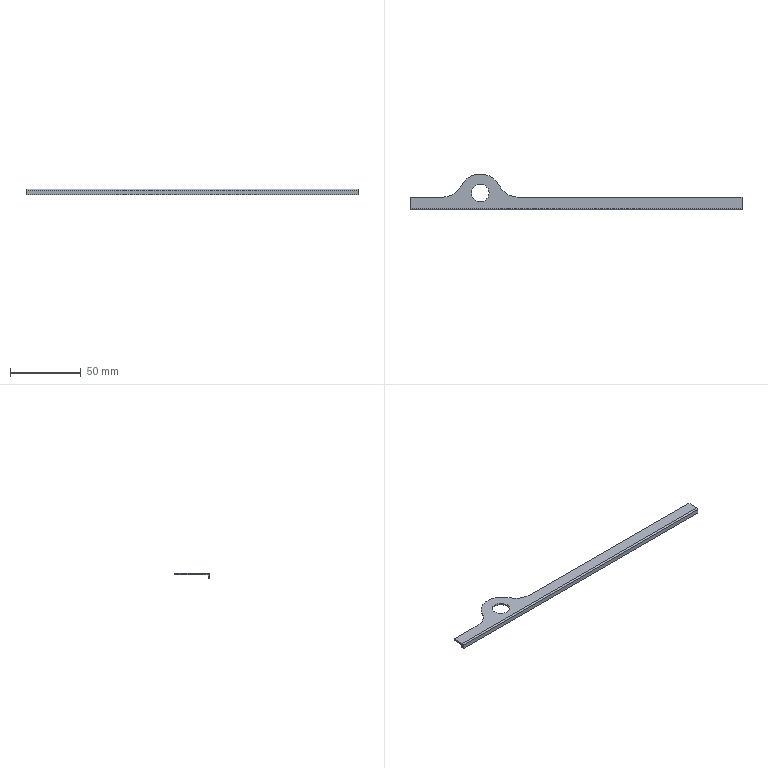Part | STEP file | gslz 2016.10.28-13_id1198_x_t | 1 solid | 14 faces | box 235 x 25.5 x 4 mm | volume 3805 mm3 | plane 9 | cylinder 5 | commonest cylinder face diameters 30 x3 2 x1 12.3 x1
STEP:
#1=CARTESIAN_POINT('',(0.,0.,0.));
#2=DIRECTION('',(0.,0.,1.));
#3=DIRECTION('',(1.,0.,0.));
#4=AXIS2_PLACEMENT_3D('',#1,#2,#3);
#5=CARTESIAN_POINT('',(1039.237,-257.,1.25));
#6=VERTEX_POINT('',#5);
#7=CARTESIAN_POINT('',(1197.655,-257.,1.25));
#8=VERTEX_POINT('',#7);
#9=CARTESIAN_POINT('',(-1199.517,-257.,1.25));
#10=DIRECTION('',(1.,0.,0.));
#11=VECTOR('',#10,1.);
#12=LINE('',#9,#11);
#13=CARTESIAN_POINT('',(1040.731,-257.,2.5));
#14=DIRECTION('',(0.,1.,0.));
#15=DIRECTION('',(-1.,0.,0.));
#16=AXIS2_PLACEMENT_3D('',#13,#14,#15);
#17=PLANE('',#16);
#18=CARTESIAN_POINT('',(2240.248,-1.25));
#19=DIRECTION('',(-1.,0.));
#20=VECTOR('',#19,1.);
#21=LINE('',#18,#20);
#22=(GEOMETRIC_REPRESENTATION_CONTEXT(2)PARAMETRIC_REPRESENTATION_CONTEXT()REPRESENTATION_CONTEXT('',''));
#23=DEFINITIONAL_REPRESENTATION('',(#21),#22);
#24=PCURVE('',#17,#23);
#25=CARTESIAN_POINT('',(-1199.517,-331.067,1.25));
#26=DIRECTION('',(0.,0.,1.));
#27=DIRECTION('',(-1.,0.,0.));
#28=AXIS2_PLACEMENT_3D('',#25,#26,#27);
#29=PLANE('',#28);
#30=CARTESIAN_POINT('',(0.,-74.067));
#31=DIRECTION('',(-1.,0.));
#32=VECTOR('',#31,1.);
#33=LINE('',#30,#32);
#34=(GEOMETRIC_REPRESENTATION_CONTEXT(2)PARAMETRIC_REPRESENTATION_CONTEXT()REPRESENTATION_CONTEXT('',''));
#35=DEFINITIONAL_REPRESENTATION('',(#33),#34);
#36=PCURVE('',#29,#35);
#37=SURFACE_CURVE('',#12,(#24,#36),.PCURVE_S1.);
#38=EDGE_CURVE('',#6,#8,#37,.T.);
#39=ORIENTED_EDGE('',*,*,#38,.T.);
#40=CARTESIAN_POINT('',(1197.655,-257.,0.));
#41=VERTEX_POINT('',#40);
#42=CARTESIAN_POINT('',(1197.655,-257.,2.5));
#43=DIRECTION('',(0.,0.,-1.));
#44=VECTOR('',#43,1.);
#45=LINE('',#42,#44);
#46=CARTESIAN_POINT('',(-156.924,0.));
#47=DIRECTION('',(0.,-1.));
#48=VECTOR('',#47,1.);
#49=LINE('',#46,#48);
#50=(GEOMETRIC_REPRESENTATION_CONTEXT(2)PARAMETRIC_REPRESENTATION_CONTEXT()REPRESENTATION_CONTEXT('',''));
#51=DEFINITIONAL_REPRESENTATION('',(#49),#50);
#52=PCURVE('',#17,#51);
#53=CARTESIAN_POINT('',(1197.655,-261.5,-0.75));
#54=DIRECTION('',(1.,0.,0.));
#55=DIRECTION('',(0.,0.,-1.));
#56=AXIS2_PLACEMENT_3D('',#53,#54,#55);
#57=PLANE('',#56);
#58=CARTESIAN_POINT('',(-3.25,4.5));
#59=DIRECTION('',(1.,0.));
#60=VECTOR('',#59,1.);
#61=LINE('',#58,#60);
#62=(GEOMETRIC_REPRESENTATION_CONTEXT(2)PARAMETRIC_REPRESENTATION_CONTEXT()REPRESENTATION_CONTEXT('',''));
#63=DEFINITIONAL_REPRESENTATION('',(#61),#62);
#64=PCURVE('',#57,#63);
#65=SURFACE_CURVE('',#45,(#52,#64),.PCURVE_S1.);
#66=EDGE_CURVE('',#8,#41,#65,.T.);
#67=ORIENTED_EDGE('',*,*,#66,.T.);
#68=CARTESIAN_POINT('',(1039.237,-257.,0.));
#69=VERTEX_POINT('',#68);
#70=CARTESIAN_POINT('',(1040.731,-257.,0.));
#71=DIRECTION('',(-1.,0.,0.));
#72=VECTOR('',#71,1.);
#73=LINE('',#70,#72);
#74=CARTESIAN_POINT('',(0.,-2.5));
#75=DIRECTION('',(1.,0.));
#76=VECTOR('',#75,1.);
#77=LINE('',#74,#76);
#78=(GEOMETRIC_REPRESENTATION_CONTEXT(2)PARAMETRIC_REPRESENTATION_CONTEXT()REPRESENTATION_CONTEXT('',''));
#79=DEFINITIONAL_REPRESENTATION('',(#77),#78);
#80=PCURVE('',#17,#79);
#81=CARTESIAN_POINT('',(-1199.517,-331.067,0.));
#82=DIRECTION('',(0.,0.,1.));
#83=DIRECTION('',(-1.,0.,0.));
#84=AXIS2_PLACEMENT_3D('',#81,#82,#83);
#85=PLANE('',#84);
#86=CARTESIAN_POINT('',(-2240.248,-74.067));
#87=DIRECTION('',(1.,0.));
#88=VECTOR('',#87,1.);
#89=LINE('',#86,#88);
#90=(GEOMETRIC_REPRESENTATION_CONTEXT(2)PARAMETRIC_REPRESENTATION_CONTEXT()REPRESENTATION_CONTEXT('',''));
#91=DEFINITIONAL_REPRESENTATION('',(#89),#90);
#92=PCURVE('',#85,#91);
#93=SURFACE_CURVE('',#73,(#80,#92),.PCURVE_S1.);
#94=EDGE_CURVE('',#41,#69,#93,.T.);
#95=ORIENTED_EDGE('',*,*,#94,.T.);
#96=CARTESIAN_POINT('',(1039.237,-257.,2.5));
#97=DIRECTION('',(0.,0.,1.));
#98=VECTOR('',#97,1.);
#99=LINE('',#96,#98);
#100=CARTESIAN_POINT('',(1.493,0.));
#101=DIRECTION('',(0.,1.));
#102=VECTOR('',#101,1.);
#103=LINE('',#100,#102);
#104=(GEOMETRIC_REPRESENTATION_CONTEXT(2)PARAMETRIC_REPRESENTATION_CONTEXT()REPRESENTATION_CONTEXT('',''));
#105=DEFINITIONAL_REPRESENTATION('',(#103),#104);
#106=PCURVE('',#17,#105);
#107=CARTESIAN_POINT('',(1039.237,-242.,2.5));
#108=DIRECTION('',(0.,0.,-1.));
#109=DIRECTION('',(1.,0.,0.));
#110=AXIS2_PLACEMENT_3D('',#107,#108,#109);
#111=CYLINDRICAL_SURFACE('',#110,15.);
#112=CARTESIAN_POINT('',(1.571,0.));
#113=DIRECTION('',(0.,-1.));
#114=VECTOR('',#113,1.);
#115=LINE('',#112,#114);
#116=(GEOMETRIC_REPRESENTATION_CONTEXT(2)PARAMETRIC_REPRESENTATION_CONTEXT()REPRESENTATION_CONTEXT('',''));
#117=DEFINITIONAL_REPRESENTATION('',(#115),#116);
#118=PCURVE('',#111,#117);
#119=SURFACE_CURVE('',#99,(#106,#118),.PCURVE_S1.);
#120=EDGE_CURVE('',#69,#6,#119,.T.);
#121=ORIENTED_EDGE('',*,*,#120,.T.);
#122=EDGE_LOOP('',(#39,#67,#95,#121));
#123=FACE_BOUND('',#122,.T.);
#124=ADVANCED_FACE('',(#123),#17,.T.);
#125=CARTESIAN_POINT('',(1006.296,-254.,1.25));
#126=VERTEX_POINT('',#125);
#127=CARTESIAN_POINT('',(1012.446,-254.,1.25));
#128=DIRECTION('',(0.,0.,1.));
#129=DIRECTION('',(-1.,0.,0.));
#130=AXIS2_PLACEMENT_3D('',#127,#128,#129);
#131=CIRCLE('',#130,6.15);
#132=CARTESIAN_POINT('',(-2211.964,-77.067));
#133=DIRECTION('',(1.,0.));
#134=AXIS2_PLACEMENT_2D('',#132,#133);
#135=CIRCLE('',#134,6.15);
#136=(GEOMETRIC_REPRESENTATION_CONTEXT(2)PARAMETRIC_REPRESENTATION_CONTEXT()REPRESENTATION_CONTEXT('',''));
#137=DEFINITIONAL_REPRESENTATION('',(#135),#136);
#138=PCURVE('',#29,#137);
#139=CARTESIAN_POINT('',(1012.446,-254.,2.5));
#140=DIRECTION('',(0.,0.,-1.));
#141=DIRECTION('',(1.,0.,0.));
#142=AXIS2_PLACEMENT_3D('',#139,#140,#141);
#143=CYLINDRICAL_SURFACE('',#142,6.15);
#144=CARTESIAN_POINT('',(9.425,1.25));
#145=DIRECTION('',(-1.,0.));
#146=VECTOR('',#145,1.);
#147=LINE('',#144,#146);
#148=(GEOMETRIC_REPRESENTATION_CONTEXT(2)PARAMETRIC_REPRESENTATION_CONTEXT()REPRESENTATION_CONTEXT('',''));
#149=DEFINITIONAL_REPRESENTATION('',(#147),#148);
#150=PCURVE('',#143,#149);
#151=SURFACE_CURVE('',#131,(#138,#150),.PCURVE_S1.);
#152=EDGE_CURVE('',#126,#126,#151,.T.);
#153=ORIENTED_EDGE('',*,*,#152,.F.);
#154=EDGE_LOOP('',(#153));
#155=FACE_BOUND('',#154,.T.);
#156=CARTESIAN_POINT('',(962.655,-265.,1.25));
#157=VERTEX_POINT('',#156);
#158=CARTESIAN_POINT('',(1197.655,-265.,1.25));
#159=VERTEX_POINT('',#158);
#160=CARTESIAN_POINT('',(1220.25,-265.,1.25));
#161=DIRECTION('',(1.,0.,0.));
#162=VECTOR('',#161,1.);
#163=LINE('',#160,#162);
#164=CARTESIAN_POINT('',(-2419.767,-66.067));
#165=DIRECTION('',(-1.,0.));
#166=VECTOR('',#165,1.);
#167=LINE('',#164,#166);
#168=(GEOMETRIC_REPRESENTATION_CONTEXT(2)PARAMETRIC_REPRESENTATION_CONTEXT()REPRESENTATION_CONTEXT('',''));
#169=DEFINITIONAL_REPRESENTATION('',(#167),#168);
#170=PCURVE('',#29,#169);
#171=CARTESIAN_POINT('',(-1199.517,-265.,0.25));
#172=DIRECTION('',(1.,0.,0.));
#173=DIRECTION('',(0.,1.,0.));
#174=AXIS2_PLACEMENT_3D('',#171,#172,#173);
#175=CYLINDRICAL_SURFACE('',#174,1.);
#176=CARTESIAN_POINT('',(1.571,2419.767));
#177=DIRECTION('',(0.,1.));
#178=VECTOR('',#177,1.);
#179=LINE('',#176,#178);
#180=(GEOMETRIC_REPRESENTATION_CONTEXT(2)PARAMETRIC_REPRESENTATION_CONTEXT()REPRESENTATION_CONTEXT('',''));
#181=DEFINITIONAL_REPRESENTATION('',(#179),#180);
#182=PCURVE('',#175,#181);
#183=SURFACE_CURVE('',#163,(#170,#182),.PCURVE_S1.);
#184=EDGE_CURVE('',#157,#159,#183,.T.);
#185=ORIENTED_EDGE('',*,*,#184,.T.);
#186=CARTESIAN_POINT('',(1197.655,-331.067,1.25));
#187=DIRECTION('',(0.,-1.,0.));
#188=VECTOR('',#187,1.);
#189=LINE('',#186,#188);
#190=CARTESIAN_POINT('',(-2397.172,0.));
#191=DIRECTION('',(0.,1.));
#192=VECTOR('',#191,1.);
#193=LINE('',#190,#192);
#194=(GEOMETRIC_REPRESENTATION_CONTEXT(2)PARAMETRIC_REPRESENTATION_CONTEXT()REPRESENTATION_CONTEXT('',''));
#195=DEFINITIONAL_REPRESENTATION('',(#193),#194);
#196=PCURVE('',#29,#195);
#197=CARTESIAN_POINT('',(-2.,-69.567));
#198=DIRECTION('',(0.,-1.));
#199=VECTOR('',#198,1.);
#200=LINE('',#197,#199);
#201=(GEOMETRIC_REPRESENTATION_CONTEXT(2)PARAMETRIC_REPRESENTATION_CONTEXT()REPRESENTATION_CONTEXT('',''));
#202=DEFINITIONAL_REPRESENTATION('',(#200),#201);
#203=PCURVE('',#57,#202);
#204=SURFACE_CURVE('',#189,(#196,#203),.PCURVE_S1.);
#205=EDGE_CURVE('',#8,#159,#204,.T.);
#206=ORIENTED_EDGE('',*,*,#205,.F.);
#207=ORIENTED_EDGE('',*,*,#38,.F.);
#208=CARTESIAN_POINT('',(1025.842,-248.75,1.25));
#209=VERTEX_POINT('',#208);
#210=CARTESIAN_POINT('',(1039.237,-242.,1.25));
#211=DIRECTION('',(0.,0.,-1.));
#212=DIRECTION('',(-1.,0.,0.));
#213=AXIS2_PLACEMENT_3D('',#210,#211,#212);
#214=CIRCLE('',#213,15.);
#215=CARTESIAN_POINT('',(-2223.754,-89.067));
#216=CARTESIAN_POINT('',(-2223.754,-115.047));
#217=CARTESIAN_POINT('',(-2246.254,-102.057));
#218=CARTESIAN_POINT('',(-2268.754,-89.067));
#219=CARTESIAN_POINT('',(-2246.254,-76.076));
#220=CARTESIAN_POINT('',(-2223.754,-63.086));
#221=CARTESIAN_POINT('',(-2223.754,-89.067));
#222=(BOUNDED_CURVE()B_SPLINE_CURVE(2,(#215,#216,#217,#218,#219,#220,#221),.UNSPECIFIED.,.T.,.F.)B_SPLINE_CURVE_WITH_KNOTS((1,2,2,2,2,1),(-2.094,0.,2.094,4.189,6.283,8.378),.UNSPECIFIED.)CURVE()GEOMETRIC_REPRESENTATION_ITEM()RATIONAL_B_SPLINE_CURVE((1.,0.5,1.,0.5,1.,0.5,1.))REPRESENTATION_ITEM(''));
#223=(GEOMETRIC_REPRESENTATION_CONTEXT(2)PARAMETRIC_REPRESENTATION_CONTEXT()REPRESENTATION_CONTEXT('',''));
#224=DEFINITIONAL_REPRESENTATION('',(#222),#223);
#225=PCURVE('',#29,#224);
#226=CARTESIAN_POINT('',(-3.142,1.25));
#227=DIRECTION('',(1.,0.));
#228=VECTOR('',#227,1.);
#229=LINE('',#226,#228);
#230=(GEOMETRIC_REPRESENTATION_CONTEXT(2)PARAMETRIC_REPRESENTATION_CONTEXT()REPRESENTATION_CONTEXT('',''));
#231=DEFINITIONAL_REPRESENTATION('',(#229),#230);
#232=PCURVE('',#111,#231);
#233=SURFACE_CURVE('',#214,(#225,#232),.PCURVE_S1.);
#234=EDGE_CURVE('',#6,#209,#233,.T.);
#235=ORIENTED_EDGE('',*,*,#234,.T.);
#236=CARTESIAN_POINT('',(999.051,-248.75,1.25));
#237=VERTEX_POINT('',#236);
#238=CARTESIAN_POINT('',(1012.446,-255.5,1.25));
#239=DIRECTION('',(0.,0.,1.));
#240=DIRECTION('',(-1.,0.,0.));
#241=AXIS2_PLACEMENT_3D('',#238,#239,#240);
#242=CIRCLE('',#241,15.);
#243=CARTESIAN_POINT('',(-2211.964,-75.567));
#244=DIRECTION('',(1.,0.));
#245=AXIS2_PLACEMENT_2D('',#243,#244);
#246=CIRCLE('',#245,15.);
#247=(GEOMETRIC_REPRESENTATION_CONTEXT(2)PARAMETRIC_REPRESENTATION_CONTEXT()REPRESENTATION_CONTEXT('',''));
#248=DEFINITIONAL_REPRESENTATION('',(#246),#247);
#249=PCURVE('',#29,#248);
#250=CARTESIAN_POINT('',(1012.446,-255.5,2.5));
#251=DIRECTION('',(0.,0.,-1.));
#252=DIRECTION('',(1.,0.,0.));
#253=AXIS2_PLACEMENT_3D('',#250,#251,#252);
#254=CYLINDRICAL_SURFACE('',#253,15.);
#255=CARTESIAN_POINT('',(9.425,1.25));
#256=DIRECTION('',(-1.,0.));
#257=VECTOR('',#256,1.);
#258=LINE('',#255,#257);
#259=(GEOMETRIC_REPRESENTATION_CONTEXT(2)PARAMETRIC_REPRESENTATION_CONTEXT()REPRESENTATION_CONTEXT('',''));
#260=DEFINITIONAL_REPRESENTATION('',(#258),#259);
#261=PCURVE('',#254,#260);
#262=SURFACE_CURVE('',#242,(#249,#261),.PCURVE_S1.);
#263=EDGE_CURVE('',#209,#237,#262,.T.);
#264=ORIENTED_EDGE('',*,*,#263,.T.);
#265=CARTESIAN_POINT('',(985.655,-257.,1.25));
#266=VERTEX_POINT('',#265);
#267=CARTESIAN_POINT('',(985.655,-242.,1.25));
#268=DIRECTION('',(0.,0.,-1.));
#269=DIRECTION('',(-1.,0.,0.));
#270=AXIS2_PLACEMENT_3D('',#267,#268,#269);
#271=CIRCLE('',#270,15.);
#272=CARTESIAN_POINT('',(-2170.173,-89.067));
#273=CARTESIAN_POINT('',(-2170.173,-115.047));
#274=CARTESIAN_POINT('',(-2192.673,-102.057));
#275=CARTESIAN_POINT('',(-2215.173,-89.067));
#276=CARTESIAN_POINT('',(-2192.673,-76.076));
#277=CARTESIAN_POINT('',(-2170.173,-63.086));
#278=CARTESIAN_POINT('',(-2170.173,-89.067));
#279=(BOUNDED_CURVE()B_SPLINE_CURVE(2,(#272,#273,#274,#275,#276,#277,#278),.UNSPECIFIED.,.T.,.F.)B_SPLINE_CURVE_WITH_KNOTS((1,2,2,2,2,1),(-2.094,0.,2.094,4.189,6.283,8.378),.UNSPECIFIED.)CURVE()GEOMETRIC_REPRESENTATION_ITEM()RATIONAL_B_SPLINE_CURVE((1.,0.5,1.,0.5,1.,0.5,1.))REPRESENTATION_ITEM(''));
#280=(GEOMETRIC_REPRESENTATION_CONTEXT(2)PARAMETRIC_REPRESENTATION_CONTEXT()REPRESENTATION_CONTEXT('',''));
#281=DEFINITIONAL_REPRESENTATION('',(#279),#280);
#282=PCURVE('',#29,#281);
#283=CARTESIAN_POINT('',(985.655,-242.,2.5));
#284=DIRECTION('',(0.,0.,-1.));
#285=DIRECTION('',(1.,0.,0.));
#286=AXIS2_PLACEMENT_3D('',#283,#284,#285);
#287=CYLINDRICAL_SURFACE('',#286,15.);
#288=CARTESIAN_POINT('',(-3.142,1.25));
#289=DIRECTION('',(1.,0.));
#290=VECTOR('',#289,1.);
#291=LINE('',#288,#290);
#292=(GEOMETRIC_REPRESENTATION_CONTEXT(2)PARAMETRIC_REPRESENTATION_CONTEXT()REPRESENTATION_CONTEXT('',''));
#293=DEFINITIONAL_REPRESENTATION('',(#291),#292);
#294=PCURVE('',#287,#293);
#295=SURFACE_CURVE('',#271,(#282,#294),.PCURVE_S1.);
#296=EDGE_CURVE('',#237,#266,#295,.T.);
#297=ORIENTED_EDGE('',*,*,#296,.T.);
#298=CARTESIAN_POINT('',(962.655,-257.,1.25));
#299=VERTEX_POINT('',#298);
#300=CARTESIAN_POINT('',(-1199.517,-257.,1.25));
#301=DIRECTION('',(1.,0.,0.));
#302=VECTOR('',#301,1.);
#303=LINE('',#300,#302);
#304=CARTESIAN_POINT('',(0.,-74.067));
#305=DIRECTION('',(-1.,0.));
#306=VECTOR('',#305,1.);
#307=LINE('',#304,#306);
#308=(GEOMETRIC_REPRESENTATION_CONTEXT(2)PARAMETRIC_REPRESENTATION_CONTEXT()REPRESENTATION_CONTEXT('',''));
#309=DEFINITIONAL_REPRESENTATION('',(#307),#308);
#310=PCURVE('',#29,#309);
#311=CARTESIAN_POINT('',(1005.291,-257.,0.));
#312=DIRECTION('',(0.,1.,0.));
#313=DIRECTION('',(0.,0.,-1.));
#314=AXIS2_PLACEMENT_3D('',#311,#312,#313);
#315=PLANE('',#314);
#316=CARTESIAN_POINT('',(-1.25,2204.808));
#317=DIRECTION('',(0.,-1.));
#318=VECTOR('',#317,1.);
#319=LINE('',#316,#318);
#320=(GEOMETRIC_REPRESENTATION_CONTEXT(2)PARAMETRIC_REPRESENTATION_CONTEXT()REPRESENTATION_CONTEXT('',''));
#321=DEFINITIONAL_REPRESENTATION('',(#319),#320);
#322=PCURVE('',#315,#321);
#323=SURFACE_CURVE('',#303,(#310,#322),.PCURVE_S1.);
#324=EDGE_CURVE('',#299,#266,#323,.T.);
#325=ORIENTED_EDGE('',*,*,#324,.F.);
#326=CARTESIAN_POINT('',(962.655,319.067,1.25));
#327=DIRECTION('',(0.,1.,0.));
#328=VECTOR('',#327,1.);
#329=LINE('',#326,#328);
#330=CARTESIAN_POINT('',(-2162.172,-650.133));
#331=DIRECTION('',(0.,-1.));
#332=VECTOR('',#331,1.);
#333=LINE('',#330,#332);
#334=(GEOMETRIC_REPRESENTATION_CONTEXT(2)PARAMETRIC_REPRESENTATION_CONTEXT()REPRESENTATION_CONTEXT('',''));
#335=DEFINITIONAL_REPRESENTATION('',(#333),#334);
#336=PCURVE('',#29,#335);
#337=CARTESIAN_POINT('',(962.655,-261.5,-0.75));
#338=DIRECTION('',(1.,0.,0.));
#339=DIRECTION('',(0.,1.,0.));
#340=AXIS2_PLACEMENT_3D('',#337,#338,#339);
#341=PLANE('',#340);
#342=CARTESIAN_POINT('',(580.567,2.));
#343=DIRECTION('',(1.,0.));
#344=VECTOR('',#343,1.);
#345=LINE('',#342,#344);
#346=(GEOMETRIC_REPRESENTATION_CONTEXT(2)PARAMETRIC_REPRESENTATION_CONTEXT()REPRESENTATION_CONTEXT('',''));
#347=DEFINITIONAL_REPRESENTATION('',(#345),#346);
#348=PCURVE('',#341,#347);
#349=SURFACE_CURVE('',#329,(#336,#348),.PCURVE_S1.);
#350=EDGE_CURVE('',#157,#299,#349,.T.);
#351=ORIENTED_EDGE('',*,*,#350,.F.);
#352=EDGE_LOOP('',(#185,#206,#207,#235,#264,#297,#325,#351));
#353=FACE_BOUND('',#352,.T.);
#354=ADVANCED_FACE('',(#155,#353),#29,.T.);
#355=CARTESIAN_POINT('',(1006.296,-254.,0.));
#356=VERTEX_POINT('',#355);
#357=CARTESIAN_POINT('',(1012.446,-254.,0.));
#358=DIRECTION('',(0.,0.,-1.));
#359=DIRECTION('',(-1.,0.,0.));
#360=AXIS2_PLACEMENT_3D('',#357,#358,#359);
#361=CIRCLE('',#360,6.15);
#362=CARTESIAN_POINT('',(-2205.814,-77.067));
#363=CARTESIAN_POINT('',(-2205.814,-87.719));
#364=CARTESIAN_POINT('',(-2215.039,-82.393));
#365=CARTESIAN_POINT('',(-2224.264,-77.067));
#366=CARTESIAN_POINT('',(-2215.039,-71.741));
#367=CARTESIAN_POINT('',(-2205.814,-66.415));
#368=CARTESIAN_POINT('',(-2205.814,-77.067));
#369=(BOUNDED_CURVE()B_SPLINE_CURVE(2,(#362,#363,#364,#365,#366,#367,#368),.UNSPECIFIED.,.T.,.F.)B_SPLINE_CURVE_WITH_KNOTS((1,2,2,2,2,1),(-2.094,0.,2.094,4.189,6.283,8.378),.UNSPECIFIED.)CURVE()GEOMETRIC_REPRESENTATION_ITEM()RATIONAL_B_SPLINE_CURVE((1.,0.5,1.,0.5,1.,0.5,1.))REPRESENTATION_ITEM(''));
#370=(GEOMETRIC_REPRESENTATION_CONTEXT(2)PARAMETRIC_REPRESENTATION_CONTEXT()REPRESENTATION_CONTEXT('',''));
#371=DEFINITIONAL_REPRESENTATION('',(#369),#370);
#372=PCURVE('',#85,#371);
#373=CARTESIAN_POINT('',(3.142,2.5));
#374=DIRECTION('',(1.,0.));
#375=VECTOR('',#374,1.);
#376=LINE('',#373,#375);
#377=(GEOMETRIC_REPRESENTATION_CONTEXT(2)PARAMETRIC_REPRESENTATION_CONTEXT()REPRESENTATION_CONTEXT('',''));
#378=DEFINITIONAL_REPRESENTATION('',(#376),#377);
#379=PCURVE('',#143,#378);
#380=SURFACE_CURVE('',#361,(#372,#379),.PCURVE_S1.);
#381=EDGE_CURVE('',#356,#356,#380,.T.);
#382=ORIENTED_EDGE('',*,*,#381,.F.);
#383=EDGE_LOOP('',(#382));
#384=FACE_BOUND('',#383,.T.);
#385=CARTESIAN_POINT('',(1197.655,-264.75,0.));
#386=VERTEX_POINT('',#385);
#387=CARTESIAN_POINT('',(1197.655,-331.067,0.));
#388=DIRECTION('',(0.,-1.,0.));
#389=VECTOR('',#388,1.);
#390=LINE('',#387,#389);
#391=CARTESIAN_POINT('',(-2397.172,0.));
#392=DIRECTION('',(0.,1.));
#393=VECTOR('',#392,1.);
#394=LINE('',#391,#393);
#395=(GEOMETRIC_REPRESENTATION_CONTEXT(2)PARAMETRIC_REPRESENTATION_CONTEXT()REPRESENTATION_CONTEXT('',''));
#396=DEFINITIONAL_REPRESENTATION('',(#394),#395);
#397=PCURVE('',#85,#396);
#398=CARTESIAN_POINT('',(-0.75,-69.567));
#399=DIRECTION('',(0.,-1.));
#400=VECTOR('',#399,1.);
#401=LINE('',#398,#400);
#402=(GEOMETRIC_REPRESENTATION_CONTEXT(2)PARAMETRIC_REPRESENTATION_CONTEXT()REPRESENTATION_CONTEXT('',''));
#403=DEFINITIONAL_REPRESENTATION('',(#401),#402);
#404=PCURVE('',#57,#403);
#405=SURFACE_CURVE('',#390,(#397,#404),.PCURVE_S1.);
#406=EDGE_CURVE('',#41,#386,#405,.T.);
#407=ORIENTED_EDGE('',*,*,#406,.T.);
#408=CARTESIAN_POINT('',(962.655,-264.75,0.));
#409=VERTEX_POINT('',#408);
#410=CARTESIAN_POINT('',(-959.851,-264.75,0.));
#411=DIRECTION('',(1.,0.,0.));
#412=VECTOR('',#411,1.);
#413=LINE('',#410,#412);
#414=CARTESIAN_POINT('',(-239.666,-66.317));
#415=DIRECTION('',(-1.,0.));
#416=VECTOR('',#415,1.);
#417=LINE('',#414,#416);
#418=(GEOMETRIC_REPRESENTATION_CONTEXT(2)PARAMETRIC_REPRESENTATION_CONTEXT()REPRESENTATION_CONTEXT('',''));
#419=DEFINITIONAL_REPRESENTATION('',(#417),#418);
#420=PCURVE('',#85,#419);
#421=CARTESIAN_POINT('',(-959.851,-264.75,-135.834));
#422=DIRECTION('',(0.,-1.,0.));
#423=DIRECTION('',(-1.,0.,0.));
#424=AXIS2_PLACEMENT_3D('',#421,#422,#423);
#425=PLANE('',#424);
#426=CARTESIAN_POINT('',(0.,-135.834));
#427=DIRECTION('',(-1.,0.));
#428=VECTOR('',#427,1.);
#429=LINE('',#426,#428);
#430=(GEOMETRIC_REPRESENTATION_CONTEXT(2)PARAMETRIC_REPRESENTATION_CONTEXT()REPRESENTATION_CONTEXT('',''));
#431=DEFINITIONAL_REPRESENTATION('',(#429),#430);
#432=PCURVE('',#425,#431);
#433=SURFACE_CURVE('',#413,(#420,#432),.PCURVE_S1.);
#434=EDGE_CURVE('',#409,#386,#433,.T.);
#435=ORIENTED_EDGE('',*,*,#434,.F.);
#436=CARTESIAN_POINT('',(962.655,-257.,0.));
#437=VERTEX_POINT('',#436);
#438=CARTESIAN_POINT('',(962.655,319.067,0.));
#439=DIRECTION('',(0.,-1.,0.));
#440=VECTOR('',#439,1.);
#441=LINE('',#438,#440);
#442=CARTESIAN_POINT('',(-2162.172,-650.133));
#443=DIRECTION('',(0.,1.));
#444=VECTOR('',#443,1.);
#445=LINE('',#442,#444);
#446=(GEOMETRIC_REPRESENTATION_CONTEXT(2)PARAMETRIC_REPRESENTATION_CONTEXT()REPRESENTATION_CONTEXT('',''));
#447=DEFINITIONAL_REPRESENTATION('',(#445),#446);
#448=PCURVE('',#85,#447);
#449=CARTESIAN_POINT('',(580.567,0.75));
#450=DIRECTION('',(-1.,0.));
#451=VECTOR('',#450,1.);
#452=LINE('',#449,#451);
#453=(GEOMETRIC_REPRESENTATION_CONTEXT(2)PARAMETRIC_REPRESENTATION_CONTEXT()REPRESENTATION_CONTEXT('',''));
#454=DEFINITIONAL_REPRESENTATION('',(#452),#453);
#455=PCURVE('',#341,#454);
#456=SURFACE_CURVE('',#441,(#448,#455),.PCURVE_S1.);
#457=EDGE_CURVE('',#437,#409,#456,.T.);
#458=ORIENTED_EDGE('',*,*,#457,.F.);
#459=CARTESIAN_POINT('',(985.655,-257.,0.));
#460=VERTEX_POINT('',#459);
#461=CARTESIAN_POINT('',(1005.291,-257.,0.));
#462=DIRECTION('',(-1.,0.,0.));
#463=VECTOR('',#462,1.);
#464=LINE('',#461,#463);
#465=CARTESIAN_POINT('',(-2204.808,-74.067));
#466=DIRECTION('',(1.,0.));
#467=VECTOR('',#466,1.);
#468=LINE('',#465,#467);
#469=(GEOMETRIC_REPRESENTATION_CONTEXT(2)PARAMETRIC_REPRESENTATION_CONTEXT()REPRESENTATION_CONTEXT('',''));
#470=DEFINITIONAL_REPRESENTATION('',(#468),#469);
#471=PCURVE('',#85,#470);
#472=CARTESIAN_POINT('',(0.,0.));
#473=DIRECTION('',(0.,1.));
#474=VECTOR('',#473,1.);
#475=LINE('',#472,#474);
#476=(GEOMETRIC_REPRESENTATION_CONTEXT(2)PARAMETRIC_REPRESENTATION_CONTEXT()REPRESENTATION_CONTEXT('',''));
#477=DEFINITIONAL_REPRESENTATION('',(#475),#476);
#478=PCURVE('',#315,#477);
#479=SURFACE_CURVE('',#464,(#471,#478),.PCURVE_S1.);
#480=EDGE_CURVE('',#460,#437,#479,.T.);
#481=ORIENTED_EDGE('',*,*,#480,.F.);
#482=CARTESIAN_POINT('',(999.051,-248.75,0.));
#483=VERTEX_POINT('',#482);
#484=CARTESIAN_POINT('',(985.655,-242.,0.));
#485=DIRECTION('',(0.,0.,1.));
#486=DIRECTION('',(-1.,0.,0.));
#487=AXIS2_PLACEMENT_3D('',#484,#485,#486);
#488=CIRCLE('',#487,15.);
#489=CARTESIAN_POINT('',(-2185.173,-89.067));
#490=DIRECTION('',(1.,0.));
#491=AXIS2_PLACEMENT_2D('',#489,#490);
#492=CIRCLE('',#491,15.);
#493=(GEOMETRIC_REPRESENTATION_CONTEXT(2)PARAMETRIC_REPRESENTATION_CONTEXT()REPRESENTATION_CONTEXT('',''));
#494=DEFINITIONAL_REPRESENTATION('',(#492),#493);
#495=PCURVE('',#85,#494);
#496=CARTESIAN_POINT('',(3.142,2.5));
#497=DIRECTION('',(-1.,0.));
#498=VECTOR('',#497,1.);
#499=LINE('',#496,#498);
#500=(GEOMETRIC_REPRESENTATION_CONTEXT(2)PARAMETRIC_REPRESENTATION_CONTEXT()REPRESENTATION_CONTEXT('',''));
#501=DEFINITIONAL_REPRESENTATION('',(#499),#500);
#502=PCURVE('',#287,#501);
#503=SURFACE_CURVE('',#488,(#495,#502),.PCURVE_S1.);
#504=EDGE_CURVE('',#460,#483,#503,.T.);
#505=ORIENTED_EDGE('',*,*,#504,.T.);
#506=CARTESIAN_POINT('',(1025.842,-248.75,0.));
#507=VERTEX_POINT('',#506);
#508=CARTESIAN_POINT('',(1012.446,-255.5,0.));
#509=DIRECTION('',(0.,0.,-1.));
#510=DIRECTION('',(-1.,0.,0.));
#511=AXIS2_PLACEMENT_3D('',#508,#509,#510);
#512=CIRCLE('',#511,15.);
#513=CARTESIAN_POINT('',(-2196.964,-75.567));
#514=CARTESIAN_POINT('',(-2196.964,-101.547));
#515=CARTESIAN_POINT('',(-2219.464,-88.557));
#516=CARTESIAN_POINT('',(-2241.964,-75.567));
#517=CARTESIAN_POINT('',(-2219.464,-62.576));
#518=CARTESIAN_POINT('',(-2196.964,-49.586));
#519=CARTESIAN_POINT('',(-2196.964,-75.567));
#520=(BOUNDED_CURVE()B_SPLINE_CURVE(2,(#513,#514,#515,#516,#517,#518,#519),.UNSPECIFIED.,.T.,.F.)B_SPLINE_CURVE_WITH_KNOTS((1,2,2,2,2,1),(-2.094,0.,2.094,4.189,6.283,8.378),.UNSPECIFIED.)CURVE()GEOMETRIC_REPRESENTATION_ITEM()RATIONAL_B_SPLINE_CURVE((1.,0.5,1.,0.5,1.,0.5,1.))REPRESENTATION_ITEM(''));
#521=(GEOMETRIC_REPRESENTATION_CONTEXT(2)PARAMETRIC_REPRESENTATION_CONTEXT()REPRESENTATION_CONTEXT('',''));
#522=DEFINITIONAL_REPRESENTATION('',(#520),#521);
#523=PCURVE('',#85,#522);
#524=CARTESIAN_POINT('',(3.142,2.5));
#525=DIRECTION('',(1.,0.));
#526=VECTOR('',#525,1.);
#527=LINE('',#524,#526);
#528=(GEOMETRIC_REPRESENTATION_CONTEXT(2)PARAMETRIC_REPRESENTATION_CONTEXT()REPRESENTATION_CONTEXT('',''));
#529=DEFINITIONAL_REPRESENTATION('',(#527),#528);
#530=PCURVE('',#254,#529);
#531=SURFACE_CURVE('',#512,(#523,#530),.PCURVE_S1.);
#532=EDGE_CURVE('',#483,#507,#531,.T.);
#533=ORIENTED_EDGE('',*,*,#532,.T.);
#534=CARTESIAN_POINT('',(1039.237,-242.,0.));
#535=DIRECTION('',(0.,0.,1.));
#536=DIRECTION('',(-1.,0.,0.));
#537=AXIS2_PLACEMENT_3D('',#534,#535,#536);
#538=CIRCLE('',#537,15.);
#539=CARTESIAN_POINT('',(-2238.754,-89.067));
#540=DIRECTION('',(1.,0.));
#541=AXIS2_PLACEMENT_2D('',#539,#540);
#542=CIRCLE('',#541,15.);
#543=(GEOMETRIC_REPRESENTATION_CONTEXT(2)PARAMETRIC_REPRESENTATION_CONTEXT()REPRESENTATION_CONTEXT('',''));
#544=DEFINITIONAL_REPRESENTATION('',(#542),#543);
#545=PCURVE('',#85,#544);
#546=CARTESIAN_POINT('',(3.142,2.5));
#547=DIRECTION('',(-1.,0.));
#548=VECTOR('',#547,1.);
#549=LINE('',#546,#548);
#550=(GEOMETRIC_REPRESENTATION_CONTEXT(2)PARAMETRIC_REPRESENTATION_CONTEXT()REPRESENTATION_CONTEXT('',''));
#551=DEFINITIONAL_REPRESENTATION('',(#549),#550);
#552=PCURVE('',#111,#551);
#553=SURFACE_CURVE('',#538,(#545,#552),.PCURVE_S1.);
#554=EDGE_CURVE('',#507,#69,#553,.T.);
#555=ORIENTED_EDGE('',*,*,#554,.T.);
#556=ORIENTED_EDGE('',*,*,#94,.F.);
#557=EDGE_LOOP('',(#407,#435,#458,#481,#505,#533,#555,#556));
#558=FACE_BOUND('',#557,.T.);
#559=ADVANCED_FACE('',(#384,#558),#85,.F.);
#560=CARTESIAN_POINT('',(1197.655,-266.,-2.75));
#561=VERTEX_POINT('',#560);
#562=CARTESIAN_POINT('',(1197.655,-264.75,-2.75));
#563=VERTEX_POINT('',#562);
#564=CARTESIAN_POINT('',(1197.655,-266.,-2.75));
#565=DIRECTION('',(0.,1.,0.));
#566=VECTOR('',#565,1.);
#567=LINE('',#564,#566);
#568=CARTESIAN_POINT('',(2314.074,-266.,-2.75));
#569=DIRECTION('',(0.,0.,1.));
#570=DIRECTION('',(1.,0.,0.));
#571=AXIS2_PLACEMENT_3D('',#568,#569,#570);
#572=PLANE('',#571);
#573=CARTESIAN_POINT('',(-1116.419,0.));
#574=DIRECTION('',(0.,1.));
#575=VECTOR('',#574,1.);
#576=LINE('',#573,#575);
#577=(GEOMETRIC_REPRESENTATION_CONTEXT(2)PARAMETRIC_REPRESENTATION_CONTEXT()REPRESENTATION_CONTEXT('',''));
#578=DEFINITIONAL_REPRESENTATION('',(#576),#577);
#579=PCURVE('',#572,#578);
#580=CARTESIAN_POINT('',(2.,-4.5));
#581=DIRECTION('',(0.,1.));
#582=VECTOR('',#581,1.);
#583=LINE('',#580,#582);
#584=(GEOMETRIC_REPRESENTATION_CONTEXT(2)PARAMETRIC_REPRESENTATION_CONTEXT()REPRESENTATION_CONTEXT('',''));
#585=DEFINITIONAL_REPRESENTATION('',(#583),#584);
#586=PCURVE('',#57,#585);
#587=SURFACE_CURVE('',#567,(#579,#586),.PCURVE_S1.);
#588=EDGE_CURVE('',#561,#563,#587,.T.);
#589=ORIENTED_EDGE('',*,*,#588,.F.);
#590=CARTESIAN_POINT('',(962.655,-266.,-2.75));
#591=VERTEX_POINT('',#590);
#592=CARTESIAN_POINT('',(2314.074,-266.,-2.75));
#593=DIRECTION('',(-1.,0.,0.));
#594=VECTOR('',#593,1.);
#595=LINE('',#592,#594);
#596=CARTESIAN_POINT('',(0.,0.));
#597=DIRECTION('',(-1.,0.));
#598=VECTOR('',#597,1.);
#599=LINE('',#596,#598);
#600=(GEOMETRIC_REPRESENTATION_CONTEXT(2)PARAMETRIC_REPRESENTATION_CONTEXT()REPRESENTATION_CONTEXT('',''));
#601=DEFINITIONAL_REPRESENTATION('',(#599),#600);
#602=PCURVE('',#572,#601);
#603=CARTESIAN_POINT('',(1052.649,-266.,0.625));
#604=DIRECTION('',(0.,-1.,0.));
#605=DIRECTION('',(-1.,0.,0.));
#606=AXIS2_PLACEMENT_3D('',#603,#604,#605);
#607=PLANE('',#606);
#608=CARTESIAN_POINT('',(-1261.425,3.375));
#609=DIRECTION('',(1.,0.));
#610=VECTOR('',#609,1.);
#611=LINE('',#608,#610);
#612=(GEOMETRIC_REPRESENTATION_CONTEXT(2)PARAMETRIC_REPRESENTATION_CONTEXT()REPRESENTATION_CONTEXT('',''));
#613=DEFINITIONAL_REPRESENTATION('',(#611),#612);
#614=PCURVE('',#607,#613);
#615=SURFACE_CURVE('',#595,(#602,#614),.PCURVE_S1.);
#616=EDGE_CURVE('',#561,#591,#615,.T.);
#617=ORIENTED_EDGE('',*,*,#616,.T.);
#618=CARTESIAN_POINT('',(962.655,-264.75,-2.75));
#619=VERTEX_POINT('',#618);
#620=CARTESIAN_POINT('',(962.655,-266.,-2.75));
#621=DIRECTION('',(0.,-1.,0.));
#622=VECTOR('',#621,1.);
#623=LINE('',#620,#622);
#624=CARTESIAN_POINT('',(-1351.419,0.));
#625=DIRECTION('',(0.,-1.));
#626=VECTOR('',#625,1.);
#627=LINE('',#624,#626);
#628=(GEOMETRIC_REPRESENTATION_CONTEXT(2)PARAMETRIC_REPRESENTATION_CONTEXT()REPRESENTATION_CONTEXT('',''));
#629=DEFINITIONAL_REPRESENTATION('',(#627),#628);
#630=PCURVE('',#572,#629);
#631=CARTESIAN_POINT('',(-4.5,-2.));
#632=DIRECTION('',(-1.,0.));
#633=VECTOR('',#632,1.);
#634=LINE('',#631,#633);
#635=(GEOMETRIC_REPRESENTATION_CONTEXT(2)PARAMETRIC_REPRESENTATION_CONTEXT()REPRESENTATION_CONTEXT('',''));
#636=DEFINITIONAL_REPRESENTATION('',(#634),#635);
#637=PCURVE('',#341,#636);
#638=SURFACE_CURVE('',#623,(#630,#637),.PCURVE_S1.);
#639=EDGE_CURVE('',#619,#591,#638,.T.);
#640=ORIENTED_EDGE('',*,*,#639,.F.);
#641=CARTESIAN_POINT('',(2314.074,-264.75,-2.75));
#642=DIRECTION('',(-1.,0.,0.));
#643=VECTOR('',#642,1.);
#644=LINE('',#641,#643);
#645=CARTESIAN_POINT('',(0.,1.25));
#646=DIRECTION('',(-1.,0.));
#647=VECTOR('',#646,1.);
#648=LINE('',#645,#647);
#649=(GEOMETRIC_REPRESENTATION_CONTEXT(2)PARAMETRIC_REPRESENTATION_CONTEXT()REPRESENTATION_CONTEXT('',''));
#650=DEFINITIONAL_REPRESENTATION('',(#648),#649);
#651=PCURVE('',#572,#650);
#652=CARTESIAN_POINT('',(-3273.925,-133.084));
#653=DIRECTION('',(1.,0.));
#654=VECTOR('',#653,1.);
#655=LINE('',#652,#654);
#656=(GEOMETRIC_REPRESENTATION_CONTEXT(2)PARAMETRIC_REPRESENTATION_CONTEXT()REPRESENTATION_CONTEXT('',''));
#657=DEFINITIONAL_REPRESENTATION('',(#655),#656);
#658=PCURVE('',#425,#657);
#659=SURFACE_CURVE('',#644,(#651,#658),.PCURVE_S1.);
#660=EDGE_CURVE('',#563,#619,#659,.T.);
#661=ORIENTED_EDGE('',*,*,#660,.F.);
#662=EDGE_LOOP('',(#589,#617,#640,#661));
#663=FACE_BOUND('',#662,.T.);
#664=ADVANCED_FACE('',(#663),#572,.F.);
#665=ORIENTED_EDGE('',*,*,#616,.F.);
#666=CARTESIAN_POINT('',(1197.655,-266.,0.25));
#667=VERTEX_POINT('',#666);
#668=CARTESIAN_POINT('',(1197.655,-266.,0.625));
#669=DIRECTION('',(0.,0.,1.));
#670=VECTOR('',#669,1.);
#671=LINE('',#668,#670);
#672=CARTESIAN_POINT('',(-145.006,0.));
#673=DIRECTION('',(0.,-1.));
#674=VECTOR('',#673,1.);
#675=LINE('',#672,#674);
#676=(GEOMETRIC_REPRESENTATION_CONTEXT(2)PARAMETRIC_REPRESENTATION_CONTEXT()REPRESENTATION_CONTEXT('',''));
#677=DEFINITIONAL_REPRESENTATION('',(#675),#676);
#678=PCURVE('',#607,#677);
#679=CARTESIAN_POINT('',(-1.375,-4.5));
#680=DIRECTION('',(-1.,0.));
#681=VECTOR('',#680,1.);
#682=LINE('',#679,#681);
#683=(GEOMETRIC_REPRESENTATION_CONTEXT(2)PARAMETRIC_REPRESENTATION_CONTEXT()REPRESENTATION_CONTEXT('',''));
#684=DEFINITIONAL_REPRESENTATION('',(#682),#683);
#685=PCURVE('',#57,#684);
#686=SURFACE_CURVE('',#671,(#678,#685),.PCURVE_S1.);
#687=EDGE_CURVE('',#561,#667,#686,.T.);
#688=ORIENTED_EDGE('',*,*,#687,.T.);
#689=CARTESIAN_POINT('',(962.655,-266.,0.25));
#690=VERTEX_POINT('',#689);
#691=CARTESIAN_POINT('',(880.149,-266.,0.25));
#692=DIRECTION('',(-1.,0.,0.));
#693=VECTOR('',#692,1.);
#694=LINE('',#691,#693);
#695=CARTESIAN_POINT('',(172.5,0.375));
#696=DIRECTION('',(1.,0.));
#697=VECTOR('',#696,1.);
#698=LINE('',#695,#697);
#699=(GEOMETRIC_REPRESENTATION_CONTEXT(2)PARAMETRIC_REPRESENTATION_CONTEXT()REPRESENTATION_CONTEXT('',''));
#700=DEFINITIONAL_REPRESENTATION('',(#698),#699);
#701=PCURVE('',#607,#700);
#702=CARTESIAN_POINT('',(3.142,2079.666));
#703=DIRECTION('',(0.,-1.));
#704=VECTOR('',#703,1.);
#705=LINE('',#702,#704);
#706=(GEOMETRIC_REPRESENTATION_CONTEXT(2)PARAMETRIC_REPRESENTATION_CONTEXT()REPRESENTATION_CONTEXT('',''));
#707=DEFINITIONAL_REPRESENTATION('',(#705),#706);
#708=PCURVE('',#175,#707);
#709=SURFACE_CURVE('',#694,(#701,#708),.PCURVE_S1.);
#710=EDGE_CURVE('',#667,#690,#709,.T.);
#711=ORIENTED_EDGE('',*,*,#710,.T.);
#712=CARTESIAN_POINT('',(962.655,-266.,0.625));
#713=DIRECTION('',(0.,0.,-1.));
#714=VECTOR('',#713,1.);
#715=LINE('',#712,#714);
#716=CARTESIAN_POINT('',(89.994,0.));
#717=DIRECTION('',(0.,1.));
#718=VECTOR('',#717,1.);
#719=LINE('',#716,#718);
#720=(GEOMETRIC_REPRESENTATION_CONTEXT(2)PARAMETRIC_REPRESENTATION_CONTEXT()REPRESENTATION_CONTEXT('',''));
#721=DEFINITIONAL_REPRESENTATION('',(#719),#720);
#722=PCURVE('',#607,#721);
#723=CARTESIAN_POINT('',(-4.5,1.375));
#724=DIRECTION('',(0.,-1.));
#725=VECTOR('',#724,1.);
#726=LINE('',#723,#725);
#727=(GEOMETRIC_REPRESENTATION_CONTEXT(2)PARAMETRIC_REPRESENTATION_CONTEXT()REPRESENTATION_CONTEXT('',''));
#728=DEFINITIONAL_REPRESENTATION('',(#726),#727);
#729=PCURVE('',#341,#728);
#730=SURFACE_CURVE('',#715,(#722,#729),.PCURVE_S1.);
#731=EDGE_CURVE('',#690,#591,#730,.T.);
#732=ORIENTED_EDGE('',*,*,#731,.T.);
#733=EDGE_LOOP('',(#665,#688,#711,#732));
#734=FACE_BOUND('',#733,.T.);
#735=ADVANCED_FACE('',(#734),#607,.T.);
#736=CARTESIAN_POINT('',(1197.655,-264.75,-135.834));
#737=DIRECTION('',(0.,0.,1.));
#738=VECTOR('',#737,1.);
#739=LINE('',#736,#738);
#740=CARTESIAN_POINT('',(-2157.506,0.));
#741=DIRECTION('',(0.,-1.));
#742=VECTOR('',#741,1.);
#743=LINE('',#740,#742);
#744=(GEOMETRIC_REPRESENTATION_CONTEXT(2)PARAMETRIC_REPRESENTATION_CONTEXT()REPRESENTATION_CONTEXT('',''));
#745=DEFINITIONAL_REPRESENTATION('',(#743),#744);
#746=PCURVE('',#425,#745);
#747=CARTESIAN_POINT('',(135.084,-3.25));
#748=DIRECTION('',(-1.,0.));
#749=VECTOR('',#748,1.);
#750=LINE('',#747,#749);
#751=(GEOMETRIC_REPRESENTATION_CONTEXT(2)PARAMETRIC_REPRESENTATION_CONTEXT()REPRESENTATION_CONTEXT('',''));
#752=DEFINITIONAL_REPRESENTATION('',(#750),#751);
#753=PCURVE('',#57,#752);
#754=SURFACE_CURVE('',#739,(#746,#753),.PCURVE_S1.);
#755=EDGE_CURVE('',#563,#386,#754,.T.);
#756=ORIENTED_EDGE('',*,*,#755,.F.);
#757=ORIENTED_EDGE('',*,*,#660,.T.);
#758=CARTESIAN_POINT('',(962.655,-264.75,-135.834));
#759=DIRECTION('',(0.,0.,-1.));
#760=VECTOR('',#759,1.);
#761=LINE('',#758,#760);
#762=CARTESIAN_POINT('',(-1922.506,0.));
#763=DIRECTION('',(0.,1.));
#764=VECTOR('',#763,1.);
#765=LINE('',#762,#764);
#766=(GEOMETRIC_REPRESENTATION_CONTEXT(2)PARAMETRIC_REPRESENTATION_CONTEXT()REPRESENTATION_CONTEXT('',''));
#767=DEFINITIONAL_REPRESENTATION('',(#765),#766);
#768=PCURVE('',#425,#767);
#769=CARTESIAN_POINT('',(-3.25,-135.084));
#770=DIRECTION('',(0.,-1.));
#771=VECTOR('',#770,1.);
#772=LINE('',#769,#771);
#773=(GEOMETRIC_REPRESENTATION_CONTEXT(2)PARAMETRIC_REPRESENTATION_CONTEXT()REPRESENTATION_CONTEXT('',''));
#774=DEFINITIONAL_REPRESENTATION('',(#772),#773);
#775=PCURVE('',#341,#774);
#776=SURFACE_CURVE('',#761,(#768,#775),.PCURVE_S1.);
#777=EDGE_CURVE('',#409,#619,#776,.T.);
#778=ORIENTED_EDGE('',*,*,#777,.F.);
#779=ORIENTED_EDGE('',*,*,#434,.T.);
#780=EDGE_LOOP('',(#756,#757,#778,#779));
#781=FACE_BOUND('',#780,.T.);
#782=ADVANCED_FACE('',(#781),#425,.F.);
#783=ORIENTED_EDGE('',*,*,#710,.F.);
#784=CARTESIAN_POINT('',(1197.655,-265.,0.25));
#785=DIRECTION('',(1.,0.,0.));
#786=DIRECTION('',(0.,0.,-1.));
#787=AXIS2_PLACEMENT_3D('',#784,#785,#786);
#788=CIRCLE('',#787,1.);
#789=CARTESIAN_POINT('',(-1.571,2397.172));
#790=DIRECTION('',(1.,0.));
#791=VECTOR('',#790,1.);
#792=LINE('',#789,#791);
#793=(GEOMETRIC_REPRESENTATION_CONTEXT(2)PARAMETRIC_REPRESENTATION_CONTEXT()REPRESENTATION_CONTEXT('',''));
#794=DEFINITIONAL_REPRESENTATION('',(#792),#793);
#795=PCURVE('',#175,#794);
#796=CARTESIAN_POINT('',(-1.,-3.5));
#797=DIRECTION('',(1.,0.));
#798=AXIS2_PLACEMENT_2D('',#796,#797);
#799=CIRCLE('',#798,1.);
#800=(GEOMETRIC_REPRESENTATION_CONTEXT(2)PARAMETRIC_REPRESENTATION_CONTEXT()REPRESENTATION_CONTEXT('',''));
#801=DEFINITIONAL_REPRESENTATION('',(#799),#800);
#802=PCURVE('',#57,#801);
#803=SURFACE_CURVE('',#788,(#795,#802),.PCURVE_S1.);
#804=EDGE_CURVE('',#159,#667,#803,.T.);
#805=ORIENTED_EDGE('',*,*,#804,.F.);
#806=ORIENTED_EDGE('',*,*,#184,.F.);
#807=CARTESIAN_POINT('',(962.655,-265.,0.25));
#808=DIRECTION('',(-1.,0.,0.));
#809=DIRECTION('',(0.,1.,0.));
#810=AXIS2_PLACEMENT_3D('',#807,#808,#809);
#811=CIRCLE('',#810,1.);
#812=CARTESIAN_POINT('',(6.283,2162.172));
#813=DIRECTION('',(-1.,0.));
#814=VECTOR('',#813,1.);
#815=LINE('',#812,#814);
#816=(GEOMETRIC_REPRESENTATION_CONTEXT(2)PARAMETRIC_REPRESENTATION_CONTEXT()REPRESENTATION_CONTEXT('',''));
#817=DEFINITIONAL_REPRESENTATION('',(#815),#816);
#818=PCURVE('',#175,#817);
#819=CARTESIAN_POINT('',(-2.5,1.));
#820=CARTESIAN_POINT('',(-2.5,-0.7321));
#821=CARTESIAN_POINT('',(-4.,0.134));
#822=CARTESIAN_POINT('',(-5.5,1.));
#823=CARTESIAN_POINT('',(-4.,1.866));
#824=CARTESIAN_POINT('',(-2.5,2.732));
#825=CARTESIAN_POINT('',(-2.5,1.));
#826=(BOUNDED_CURVE()B_SPLINE_CURVE(2,(#819,#820,#821,#822,#823,#824,#825),.UNSPECIFIED.,.T.,.F.)B_SPLINE_CURVE_WITH_KNOTS((1,2,2,2,2,1),(-2.094,0.,2.094,4.189,6.283,8.378),.UNSPECIFIED.)CURVE()GEOMETRIC_REPRESENTATION_ITEM()RATIONAL_B_SPLINE_CURVE((1.,0.5,1.,0.5,1.,0.5,1.))REPRESENTATION_ITEM(''));
#827=(GEOMETRIC_REPRESENTATION_CONTEXT(2)PARAMETRIC_REPRESENTATION_CONTEXT()REPRESENTATION_CONTEXT('',''));
#828=DEFINITIONAL_REPRESENTATION('',(#826),#827);
#829=PCURVE('',#341,#828);
#830=SURFACE_CURVE('',#811,(#818,#829),.PCURVE_S1.);
#831=EDGE_CURVE('',#690,#157,#830,.T.);
#832=ORIENTED_EDGE('',*,*,#831,.F.);
#833=EDGE_LOOP('',(#783,#805,#806,#832));
#834=FACE_BOUND('',#833,.T.);
#835=ADVANCED_FACE('',(#834),#175,.T.);
#836=ORIENTED_EDGE('',*,*,#152,.F.);
#837=CARTESIAN_POINT('',(1006.296,-254.,1.25));
#838=CARTESIAN_POINT('',(1006.296,-254.,0.));
#839=B_SPLINE_CURVE_WITH_KNOTS('',1,(#837,#838),.UNSPECIFIED.,.F.,.F.,(2,2),(1.25,2.5),.PIECEWISE_BEZIER_KNOTS.);
#840=CARTESIAN_POINT('',(9.425,0.));
#841=DIRECTION('',(0.,1.));
#842=VECTOR('',#841,1.);
#843=LINE('',#840,#842);
#844=(GEOMETRIC_REPRESENTATION_CONTEXT(2)PARAMETRIC_REPRESENTATION_CONTEXT()REPRESENTATION_CONTEXT('',''));
#845=DEFINITIONAL_REPRESENTATION('',(#843),#844);
#846=PCURVE('',#143,#845);
#847=CARTESIAN_POINT('',(3.142,0.));
#848=DIRECTION('',(0.,1.));
#849=VECTOR('',#848,1.);
#850=LINE('',#847,#849);
#851=(GEOMETRIC_REPRESENTATION_CONTEXT(2)PARAMETRIC_REPRESENTATION_CONTEXT()REPRESENTATION_CONTEXT('',''));
#852=DEFINITIONAL_REPRESENTATION('',(#850),#851);
#853=PCURVE('',#143,#852);
#854=SEAM_CURVE('',#839,(#846,#853),.PCURVE_S1.);
#855=EDGE_CURVE('',#126,#356,#854,.T.);
#856=ORIENTED_EDGE('',*,*,#855,.T.);
#857=ORIENTED_EDGE('',*,*,#381,.F.);
#858=ORIENTED_EDGE('',*,*,#855,.F.);
#859=EDGE_LOOP('',(#836,#856,#857,#858));
#860=FACE_BOUND('',#859,.F.);
#861=ADVANCED_FACE('',(#860),#143,.F.);
#862=ORIENTED_EDGE('',*,*,#480,.T.);
#863=CARTESIAN_POINT('',(962.655,-257.,2.5));
#864=DIRECTION('',(0.,0.,1.));
#865=VECTOR('',#864,1.);
#866=LINE('',#863,#865);
#867=CARTESIAN_POINT('',(-2.5,42.636));
#868=DIRECTION('',(-1.,0.));
#869=VECTOR('',#868,1.);
#870=LINE('',#867,#869);
#871=(GEOMETRIC_REPRESENTATION_CONTEXT(2)PARAMETRIC_REPRESENTATION_CONTEXT()REPRESENTATION_CONTEXT('',''));
#872=DEFINITIONAL_REPRESENTATION('',(#870),#871);
#873=PCURVE('',#315,#872);
#874=CARTESIAN_POINT('',(4.5,3.25));
#875=DIRECTION('',(0.,1.));
#876=VECTOR('',#875,1.);
#877=LINE('',#874,#876);
#878=(GEOMETRIC_REPRESENTATION_CONTEXT(2)PARAMETRIC_REPRESENTATION_CONTEXT()REPRESENTATION_CONTEXT('',''));
#879=DEFINITIONAL_REPRESENTATION('',(#877),#878);
#880=PCURVE('',#341,#879);
#881=SURFACE_CURVE('',#866,(#873,#880),.PCURVE_S1.);
#882=EDGE_CURVE('',#437,#299,#881,.T.);
#883=ORIENTED_EDGE('',*,*,#882,.T.);
#884=ORIENTED_EDGE('',*,*,#324,.T.);
#885=CARTESIAN_POINT('',(985.655,-257.,2.5));
#886=DIRECTION('',(0.,0.,1.));
#887=VECTOR('',#886,1.);
#888=LINE('',#885,#887);
#889=CARTESIAN_POINT('',(-2.5,19.635));
#890=DIRECTION('',(-1.,0.));
#891=VECTOR('',#890,1.);
#892=LINE('',#889,#891);
#893=(GEOMETRIC_REPRESENTATION_CONTEXT(2)PARAMETRIC_REPRESENTATION_CONTEXT()REPRESENTATION_CONTEXT('',''));
#894=DEFINITIONAL_REPRESENTATION('',(#892),#893);
#895=PCURVE('',#315,#894);
#896=CARTESIAN_POINT('',(1.571,0.));
#897=DIRECTION('',(0.,-1.));
#898=VECTOR('',#897,1.);
#899=LINE('',#896,#898);
#900=(GEOMETRIC_REPRESENTATION_CONTEXT(2)PARAMETRIC_REPRESENTATION_CONTEXT()REPRESENTATION_CONTEXT('',''));
#901=DEFINITIONAL_REPRESENTATION('',(#899),#900);
#902=PCURVE('',#287,#901);
#903=SURFACE_CURVE('',#888,(#895,#902),.PCURVE_S1.);
#904=EDGE_CURVE('',#460,#266,#903,.T.);
#905=ORIENTED_EDGE('',*,*,#904,.F.);
#906=EDGE_LOOP('',(#862,#883,#884,#905));
#907=FACE_BOUND('',#906,.T.);
#908=ADVANCED_FACE('',(#907),#315,.T.);
#909=ORIENTED_EDGE('',*,*,#532,.F.);
#910=CARTESIAN_POINT('',(999.051,-248.75,0.625));
#911=DIRECTION('',(0.,0.,1.));
#912=VECTOR('',#911,1.);
#913=LINE('',#910,#912);
#914=CARTESIAN_POINT('',(3.608,1.875));
#915=DIRECTION('',(0.,-1.));
#916=VECTOR('',#915,1.);
#917=LINE('',#914,#916);
#918=(GEOMETRIC_REPRESENTATION_CONTEXT(2)PARAMETRIC_REPRESENTATION_CONTEXT()REPRESENTATION_CONTEXT('',''));
#919=DEFINITIONAL_REPRESENTATION('',(#917),#918);
#920=PCURVE('',#254,#919);
#921=CARTESIAN_POINT('',(0.4668,1.875));
#922=DIRECTION('',(0.,-1.));
#923=VECTOR('',#922,1.);
#924=LINE('',#921,#923);
#925=(GEOMETRIC_REPRESENTATION_CONTEXT(2)PARAMETRIC_REPRESENTATION_CONTEXT()REPRESENTATION_CONTEXT('',''));
#926=DEFINITIONAL_REPRESENTATION('',(#924),#925);
#927=PCURVE('',#287,#926);
#928=SURFACE_CURVE('',#913,(#920,#927),.PCURVE_S1.);
#929=EDGE_CURVE('',#483,#237,#928,.T.);
#930=ORIENTED_EDGE('',*,*,#929,.T.);
#931=ORIENTED_EDGE('',*,*,#263,.F.);
#932=CARTESIAN_POINT('',(1025.842,-248.75,0.625));
#933=DIRECTION('',(0.,0.,1.));
#934=VECTOR('',#933,1.);
#935=LINE('',#932,#934);
#936=CARTESIAN_POINT('',(5.816,1.875));
#937=DIRECTION('',(0.,-1.));
#938=VECTOR('',#937,1.);
#939=LINE('',#936,#938);
#940=(GEOMETRIC_REPRESENTATION_CONTEXT(2)PARAMETRIC_REPRESENTATION_CONTEXT()REPRESENTATION_CONTEXT('',''));
#941=DEFINITIONAL_REPRESENTATION('',(#939),#940);
#942=PCURVE('',#254,#941);
#943=CARTESIAN_POINT('',(2.675,1.875));
#944=DIRECTION('',(0.,-1.));
#945=VECTOR('',#944,1.);
#946=LINE('',#943,#945);
#947=(GEOMETRIC_REPRESENTATION_CONTEXT(2)PARAMETRIC_REPRESENTATION_CONTEXT()REPRESENTATION_CONTEXT('',''));
#948=DEFINITIONAL_REPRESENTATION('',(#946),#947);
#949=PCURVE('',#111,#948);
#950=SURFACE_CURVE('',#935,(#942,#949),.PCURVE_S1.);
#951=EDGE_CURVE('',#507,#209,#950,.T.);
#952=ORIENTED_EDGE('',*,*,#951,.F.);
#953=EDGE_LOOP('',(#909,#930,#931,#952));
#954=FACE_BOUND('',#953,.T.);
#955=ADVANCED_FACE('',(#954),#254,.T.);
#956=ORIENTED_EDGE('',*,*,#296,.T.);
#957=ORIENTED_EDGE('',*,*,#904,.F.);
#958=ORIENTED_EDGE('',*,*,#504,.T.);
#959=ORIENTED_EDGE('',*,*,#929,.T.);
#960=EDGE_LOOP('',(#956,#957,#958,#959));
#961=FACE_BOUND('',#960,.F.);
#962=ADVANCED_FACE('',(#961),#287,.F.);
#963=ORIENTED_EDGE('',*,*,#234,.T.);
#964=ORIENTED_EDGE('',*,*,#951,.F.);
#965=ORIENTED_EDGE('',*,*,#554,.T.);
#966=ORIENTED_EDGE('',*,*,#120,.T.);
#967=EDGE_LOOP('',(#963,#964,#965,#966));
#968=FACE_BOUND('',#967,.F.);
#969=ADVANCED_FACE('',(#968),#111,.F.);
#970=ORIENTED_EDGE('',*,*,#457,.T.);
#971=ORIENTED_EDGE('',*,*,#777,.T.);
#972=ORIENTED_EDGE('',*,*,#639,.T.);
#973=ORIENTED_EDGE('',*,*,#731,.F.);
#974=ORIENTED_EDGE('',*,*,#831,.T.);
#975=ORIENTED_EDGE('',*,*,#350,.T.);
#976=ORIENTED_EDGE('',*,*,#882,.F.);
#977=EDGE_LOOP('',(#970,#971,#972,#973,#974,#975,#976));
#978=FACE_BOUND('',#977,.T.);
#979=ADVANCED_FACE('',(#978),#341,.F.);
#980=ORIENTED_EDGE('',*,*,#755,.T.);
#981=ORIENTED_EDGE('',*,*,#406,.F.);
#982=ORIENTED_EDGE('',*,*,#66,.F.);
#983=ORIENTED_EDGE('',*,*,#205,.T.);
#984=ORIENTED_EDGE('',*,*,#804,.T.);
#985=ORIENTED_EDGE('',*,*,#687,.F.);
#986=ORIENTED_EDGE('',*,*,#588,.T.);
#987=EDGE_LOOP('',(#980,#981,#982,#983,#984,#985,#986));
#988=FACE_BOUND('',#987,.T.);
#989=ADVANCED_FACE('',(#988),#57,.T.);
#990=CLOSED_SHELL('',(#124,#354,#559,#664,#735,#782,#835,#861,#908,#955,#962,#969,#979,#989));
#991=MANIFOLD_SOLID_BREP('',#990);
#992=(LENGTH_UNIT()NAMED_UNIT(*)SI_UNIT(.MILLI.,.METRE.));
#993=UNCERTAINTY_MEASURE_WITH_UNIT(LENGTH_MEASURE(0.000001),#992,'','');
#994=(NAMED_UNIT(*)PLANE_ANGLE_UNIT()SI_UNIT($,.RADIAN.));
#995=(NAMED_UNIT(*)SI_UNIT($,.STERADIAN.)SOLID_ANGLE_UNIT());
#996=(GEOMETRIC_REPRESENTATION_CONTEXT(3)GLOBAL_UNCERTAINTY_ASSIGNED_CONTEXT((#993))GLOBAL_UNIT_ASSIGNED_CONTEXT((#992,#994,#995))REPRESENTATION_CONTEXT('',''));
#997=ADVANCED_BREP_SHAPE_REPRESENTATION('',(#4,#991),#996);